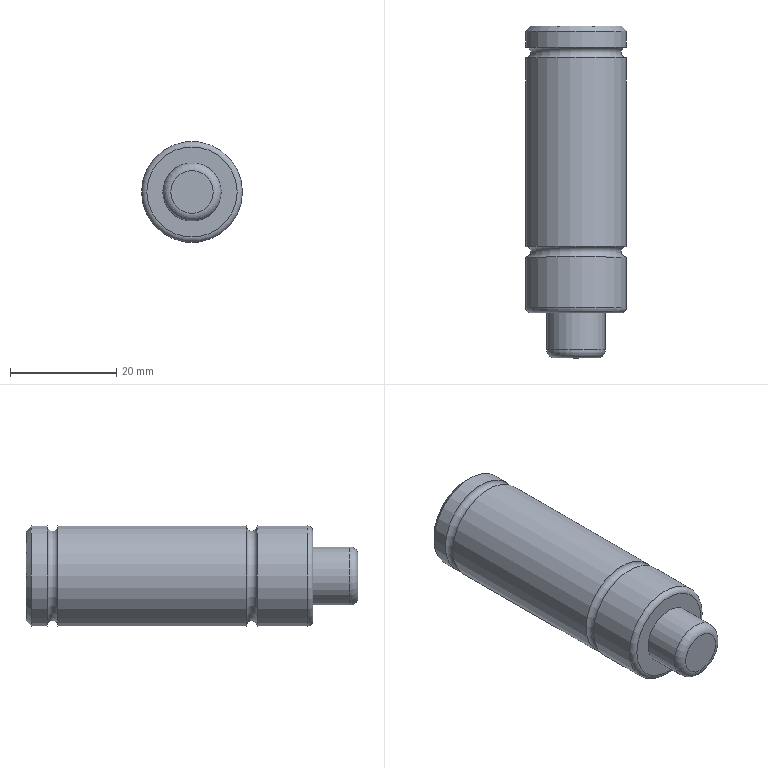Part | STEP file | 1_id602_x_t | 1 solid | 14 faces | box 19 x 62.5 x 19 mm | volume 15480 mm3 | cylinder 5 | torus 4 | plane 3 | cone 2 | commonest cylinder face diameters 19 x3 5 x1 11 x1
STEP:
#1=CARTESIAN_POINT('',(0.,0.,0.));
#2=DIRECTION('',(0.,0.,1.));
#3=DIRECTION('',(1.,0.,0.));
#4=AXIS2_PLACEMENT_3D('',#1,#2,#3);
#5=CARTESIAN_POINT('',(747.425,262.37,-108.684));
#6=VERTEX_POINT('',#5);
#7=CARTESIAN_POINT('',(752.425,262.37,-108.684));
#8=VERTEX_POINT('',#7);
#9=CARTESIAN_POINT('',(749.925,262.37,-108.684));
#10=DIRECTION('',(0.,1.,0.));
#11=DIRECTION('',(1.,0.,0.));
#12=AXIS2_PLACEMENT_3D('',#9,#10,#11);
#13=CIRCLE('',#12,2.5);
#14=CARTESIAN_POINT('',(749.925,261.669,-108.684));
#15=DIRECTION('',(0.,1.,0.));
#16=DIRECTION('',(-1.,0.,0.));
#17=AXIS2_PLACEMENT_3D('',#14,#15,#16);
#18=CONICAL_SURFACE('',#17,1.285,1.047);
#19=CARTESIAN_POINT('',(-3.142,0.7013));
#20=DIRECTION('',(1.,0.));
#21=VECTOR('',#20,1.);
#22=LINE('',#19,#21);
#23=(GEOMETRIC_REPRESENTATION_CONTEXT(2)PARAMETRIC_REPRESENTATION_CONTEXT()REPRESENTATION_CONTEXT('',''));
#24=DEFINITIONAL_REPRESENTATION('',(#22),#23);
#25=PCURVE('',#18,#24);
#26=CARTESIAN_POINT('',(749.925,262.37,-108.684));
#27=DIRECTION('',(0.,-1.,0.));
#28=DIRECTION('',(-1.,0.,0.));
#29=AXIS2_PLACEMENT_3D('',#26,#27,#28);
#30=CYLINDRICAL_SURFACE('',#29,2.5);
#31=CARTESIAN_POINT('',(9.425,0.));
#32=DIRECTION('',(-1.,0.));
#33=VECTOR('',#32,1.);
#34=LINE('',#31,#33);
#35=(GEOMETRIC_REPRESENTATION_CONTEXT(2)PARAMETRIC_REPRESENTATION_CONTEXT()REPRESENTATION_CONTEXT('',''));
#36=DEFINITIONAL_REPRESENTATION('',(#34),#35);
#37=PCURVE('',#30,#36);
#38=SURFACE_CURVE('',#13,(#25,#37),.PCURVE_S1.);
#39=EDGE_CURVE('',#6,#8,#38,.T.);
#40=ORIENTED_EDGE('',*,*,#39,.F.);
#41=CARTESIAN_POINT('',(749.925,260.927,-108.684));
#42=VERTEX_POINT('',#41);
#43=CARTESIAN_POINT('',(749.925,260.927,-108.684));
#44=CARTESIAN_POINT('',(747.425,262.37,-108.684));
#45=B_SPLINE_CURVE_WITH_KNOTS('',1,(#43,#44),.UNSPECIFIED.,.F.,.F.,(2,2),(-1.484,1.403),.PIECEWISE_BEZIER_KNOTS.);
#46=CARTESIAN_POINT('',(0.,0.));
#47=DIRECTION('',(0.,1.));
#48=VECTOR('',#47,1.);
#49=LINE('',#46,#48);
#50=(GEOMETRIC_REPRESENTATION_CONTEXT(2)PARAMETRIC_REPRESENTATION_CONTEXT()REPRESENTATION_CONTEXT('',''));
#51=DEFINITIONAL_REPRESENTATION('',(#49),#50);
#52=PCURVE('',#18,#51);
#53=CARTESIAN_POINT('',(6.283,0.));
#54=DIRECTION('',(0.,1.));
#55=VECTOR('',#54,1.);
#56=LINE('',#53,#55);
#57=(GEOMETRIC_REPRESENTATION_CONTEXT(2)PARAMETRIC_REPRESENTATION_CONTEXT()REPRESENTATION_CONTEXT('',''));
#58=DEFINITIONAL_REPRESENTATION('',(#56),#57);
#59=PCURVE('',#18,#58);
#60=SEAM_CURVE('',#45,(#52,#59),.PCURVE_S1.);
#61=EDGE_CURVE('',#42,#6,#60,.T.);
#62=ORIENTED_EDGE('',*,*,#61,.F.);
#63=ORIENTED_EDGE('',*,*,#61,.T.);
#64=CARTESIAN_POINT('',(749.925,262.37,-108.684));
#65=DIRECTION('',(0.,1.,0.));
#66=DIRECTION('',(1.,0.,0.));
#67=AXIS2_PLACEMENT_3D('',#64,#65,#66);
#68=CIRCLE('',#67,2.5);
#69=CARTESIAN_POINT('',(3.142,0.7013));
#70=DIRECTION('',(1.,0.));
#71=VECTOR('',#70,1.);
#72=LINE('',#69,#71);
#73=(GEOMETRIC_REPRESENTATION_CONTEXT(2)PARAMETRIC_REPRESENTATION_CONTEXT()REPRESENTATION_CONTEXT('',''));
#74=DEFINITIONAL_REPRESENTATION('',(#72),#73);
#75=PCURVE('',#18,#74);
#76=CARTESIAN_POINT('',(3.142,0.));
#77=DIRECTION('',(-1.,0.));
#78=VECTOR('',#77,1.);
#79=LINE('',#76,#78);
#80=(GEOMETRIC_REPRESENTATION_CONTEXT(2)PARAMETRIC_REPRESENTATION_CONTEXT()REPRESENTATION_CONTEXT('',''));
#81=DEFINITIONAL_REPRESENTATION('',(#79),#80);
#82=PCURVE('',#30,#81);
#83=SURFACE_CURVE('',#68,(#75,#82),.PCURVE_S1.);
#84=EDGE_CURVE('',#8,#6,#83,.T.);
#85=ORIENTED_EDGE('',*,*,#84,.F.);
#86=EDGE_LOOP('',(#40,#62,#63,#85));
#87=FACE_BOUND('',#86,.F.);
#88=ADVANCED_FACE('',(#87),#18,.F.);
#89=ORIENTED_EDGE('',*,*,#39,.T.);
#90=ORIENTED_EDGE('',*,*,#84,.T.);
#91=CARTESIAN_POINT('',(747.425,282.37,-108.684));
#92=VERTEX_POINT('',#91);
#93=CARTESIAN_POINT('',(747.425,282.37,-108.684));
#94=CARTESIAN_POINT('',(747.425,262.37,-108.684));
#95=B_SPLINE_CURVE_WITH_KNOTS('',1,(#93,#94),.UNSPECIFIED.,.F.,.F.,(2,2),(-20.,0.),.PIECEWISE_BEZIER_KNOTS.);
#96=CARTESIAN_POINT('',(0.,0.));
#97=DIRECTION('',(0.,1.));
#98=VECTOR('',#97,1.);
#99=LINE('',#96,#98);
#100=(GEOMETRIC_REPRESENTATION_CONTEXT(2)PARAMETRIC_REPRESENTATION_CONTEXT()REPRESENTATION_CONTEXT('',''));
#101=DEFINITIONAL_REPRESENTATION('',(#99),#100);
#102=PCURVE('',#30,#101);
#103=CARTESIAN_POINT('',(6.283,0.));
#104=DIRECTION('',(0.,1.));
#105=VECTOR('',#104,1.);
#106=LINE('',#103,#105);
#107=(GEOMETRIC_REPRESENTATION_CONTEXT(2)PARAMETRIC_REPRESENTATION_CONTEXT()REPRESENTATION_CONTEXT('',''));
#108=DEFINITIONAL_REPRESENTATION('',(#106),#107);
#109=PCURVE('',#30,#108);
#110=SEAM_CURVE('',#95,(#102,#109),.PCURVE_S1.);
#111=EDGE_CURVE('',#92,#6,#110,.T.);
#112=ORIENTED_EDGE('',*,*,#111,.F.);
#113=CARTESIAN_POINT('',(749.925,282.37,-108.684));
#114=DIRECTION('',(0.,-1.,0.));
#115=DIRECTION('',(-1.,0.,0.));
#116=AXIS2_PLACEMENT_3D('',#113,#114,#115);
#117=CIRCLE('',#116,2.5);
#118=CARTESIAN_POINT('',(0.,-20.));
#119=DIRECTION('',(1.,0.));
#120=VECTOR('',#119,1.);
#121=LINE('',#118,#120);
#122=(GEOMETRIC_REPRESENTATION_CONTEXT(2)PARAMETRIC_REPRESENTATION_CONTEXT()REPRESENTATION_CONTEXT('',''));
#123=DEFINITIONAL_REPRESENTATION('',(#121),#122);
#124=PCURVE('',#30,#123);
#125=CARTESIAN_POINT('',(749.925,282.37,-100.184));
#126=DIRECTION('',(0.,-1.,0.));
#127=DIRECTION('',(-1.,0.,0.));
#128=AXIS2_PLACEMENT_3D('',#125,#126,#127);
#129=PLANE('',#128);
#130=CARTESIAN_POINT('',(0.,8.5));
#131=DIRECTION('',(1.,0.));
#132=AXIS2_PLACEMENT_2D('',#130,#131);
#133=CIRCLE('',#132,2.5);
#134=(GEOMETRIC_REPRESENTATION_CONTEXT(2)PARAMETRIC_REPRESENTATION_CONTEXT()REPRESENTATION_CONTEXT('',''));
#135=DEFINITIONAL_REPRESENTATION('',(#133),#134);
#136=PCURVE('',#129,#135);
#137=SURFACE_CURVE('',#117,(#124,#136),.PCURVE_S1.);
#138=EDGE_CURVE('',#92,#92,#137,.T.);
#139=ORIENTED_EDGE('',*,*,#138,.T.);
#140=ORIENTED_EDGE('',*,*,#111,.T.);
#141=EDGE_LOOP('',(#89,#90,#112,#139,#140));
#142=FACE_BOUND('',#141,.F.);
#143=ADVANCED_FACE('',(#142),#30,.F.);
#144=CARTESIAN_POINT('',(758.425,282.37,-108.684));
#145=VERTEX_POINT('',#144);
#146=CARTESIAN_POINT('',(749.925,282.37,-108.684));
#147=DIRECTION('',(0.,1.,0.));
#148=DIRECTION('',(1.,0.,0.));
#149=AXIS2_PLACEMENT_3D('',#146,#147,#148);
#150=CIRCLE('',#149,8.5);
#151=CARTESIAN_POINT('',(-8.5,8.5));
#152=CARTESIAN_POINT('',(-8.5,23.222));
#153=CARTESIAN_POINT('',(4.25,15.861));
#154=CARTESIAN_POINT('',(17.,8.5));
#155=CARTESIAN_POINT('',(4.25,1.139));
#156=CARTESIAN_POINT('',(-8.5,-6.222));
#157=CARTESIAN_POINT('',(-8.5,8.5));
#158=(BOUNDED_CURVE()B_SPLINE_CURVE(2,(#151,#152,#153,#154,#155,#156,#157),.UNSPECIFIED.,.T.,.F.)B_SPLINE_CURVE_WITH_KNOTS((1,2,2,2,2,1),(-2.094,0.,2.094,4.189,6.283,8.378),.UNSPECIFIED.)CURVE()GEOMETRIC_REPRESENTATION_ITEM()RATIONAL_B_SPLINE_CURVE((1.,0.5,1.,0.5,1.,0.5,1.))REPRESENTATION_ITEM(''));
#159=(GEOMETRIC_REPRESENTATION_CONTEXT(2)PARAMETRIC_REPRESENTATION_CONTEXT()REPRESENTATION_CONTEXT('',''));
#160=DEFINITIONAL_REPRESENTATION('',(#158),#159);
#161=PCURVE('',#129,#160);
#162=CARTESIAN_POINT('',(749.925,281.87,-108.684));
#163=DIRECTION('',(0.,-1.,0.));
#164=DIRECTION('',(1.,0.,0.));
#165=AXIS2_PLACEMENT_3D('',#162,#163,#164);
#166=CONICAL_SURFACE('',#165,9.,0.7854);
#167=CARTESIAN_POINT('',(6.283,-0.5));
#168=DIRECTION('',(-1.,0.));
#169=VECTOR('',#168,1.);
#170=LINE('',#167,#169);
#171=(GEOMETRIC_REPRESENTATION_CONTEXT(2)PARAMETRIC_REPRESENTATION_CONTEXT()REPRESENTATION_CONTEXT('',''));
#172=DEFINITIONAL_REPRESENTATION('',(#170),#171);
#173=PCURVE('',#166,#172);
#174=SURFACE_CURVE('',#150,(#161,#173),.PCURVE_S1.);
#175=EDGE_CURVE('',#145,#145,#174,.T.);
#176=ORIENTED_EDGE('',*,*,#175,.T.);
#177=EDGE_LOOP('',(#176));
#178=FACE_BOUND('',#177,.T.);
#179=ORIENTED_EDGE('',*,*,#138,.T.);
#180=EDGE_LOOP('',(#179));
#181=FACE_BOUND('',#180,.T.);
#182=ADVANCED_FACE('',(#178,#181),#129,.F.);
#183=CARTESIAN_POINT('',(759.425,281.37,-108.684));
#184=VERTEX_POINT('',#183);
#185=CARTESIAN_POINT('',(740.425,281.37,-108.684));
#186=VERTEX_POINT('',#185);
#187=CARTESIAN_POINT('',(749.925,281.37,-108.684));
#188=DIRECTION('',(0.,1.,0.));
#189=DIRECTION('',(1.,0.,0.));
#190=AXIS2_PLACEMENT_3D('',#187,#188,#189);
#191=CIRCLE('',#190,9.5);
#192=CARTESIAN_POINT('',(6.283,0.5));
#193=DIRECTION('',(-1.,0.));
#194=VECTOR('',#193,1.);
#195=LINE('',#192,#194);
#196=(GEOMETRIC_REPRESENTATION_CONTEXT(2)PARAMETRIC_REPRESENTATION_CONTEXT()REPRESENTATION_CONTEXT('',''));
#197=DEFINITIONAL_REPRESENTATION('',(#195),#196);
#198=PCURVE('',#166,#197);
#199=CARTESIAN_POINT('',(749.925,228.37,-108.684));
#200=DIRECTION('',(0.,-1.,0.));
#201=DIRECTION('',(-1.,0.,0.));
#202=AXIS2_PLACEMENT_3D('',#199,#200,#201);
#203=CYLINDRICAL_SURFACE('',#202,9.5);
#204=CARTESIAN_POINT('',(3.142,-53.));
#205=DIRECTION('',(-1.,0.));
#206=VECTOR('',#205,1.);
#207=LINE('',#204,#206);
#208=(GEOMETRIC_REPRESENTATION_CONTEXT(2)PARAMETRIC_REPRESENTATION_CONTEXT()REPRESENTATION_CONTEXT('',''));
#209=DEFINITIONAL_REPRESENTATION('',(#207),#208);
#210=PCURVE('',#203,#209);
#211=SURFACE_CURVE('',#191,(#198,#210),.PCURVE_S1.);
#212=EDGE_CURVE('',#184,#186,#211,.T.);
#213=ORIENTED_EDGE('',*,*,#212,.T.);
#214=CARTESIAN_POINT('',(749.925,281.37,-108.684));
#215=DIRECTION('',(0.,1.,0.));
#216=DIRECTION('',(1.,0.,0.));
#217=AXIS2_PLACEMENT_3D('',#214,#215,#216);
#218=CIRCLE('',#217,9.5);
#219=CARTESIAN_POINT('',(6.283,0.5));
#220=DIRECTION('',(-1.,0.));
#221=VECTOR('',#220,1.);
#222=LINE('',#219,#221);
#223=(GEOMETRIC_REPRESENTATION_CONTEXT(2)PARAMETRIC_REPRESENTATION_CONTEXT()REPRESENTATION_CONTEXT('',''));
#224=DEFINITIONAL_REPRESENTATION('',(#222),#223);
#225=PCURVE('',#166,#224);
#226=CARTESIAN_POINT('',(9.425,-53.));
#227=DIRECTION('',(-1.,0.));
#228=VECTOR('',#227,1.);
#229=LINE('',#226,#228);
#230=(GEOMETRIC_REPRESENTATION_CONTEXT(2)PARAMETRIC_REPRESENTATION_CONTEXT()REPRESENTATION_CONTEXT('',''));
#231=DEFINITIONAL_REPRESENTATION('',(#229),#230);
#232=PCURVE('',#203,#231);
#233=SURFACE_CURVE('',#218,(#225,#232),.PCURVE_S1.);
#234=EDGE_CURVE('',#186,#184,#233,.T.);
#235=ORIENTED_EDGE('',*,*,#234,.T.);
#236=CARTESIAN_POINT('',(758.425,282.37,-108.684));
#237=CARTESIAN_POINT('',(759.425,281.37,-108.684));
#238=B_SPLINE_CURVE_WITH_KNOTS('',1,(#236,#237),.UNSPECIFIED.,.F.,.F.,(2,2),(-0.7071,0.7071),.PIECEWISE_BEZIER_KNOTS.);
#239=CARTESIAN_POINT('',(0.,0.));
#240=DIRECTION('',(0.,1.));
#241=VECTOR('',#240,1.);
#242=LINE('',#239,#241);
#243=(GEOMETRIC_REPRESENTATION_CONTEXT(2)PARAMETRIC_REPRESENTATION_CONTEXT()REPRESENTATION_CONTEXT('',''));
#244=DEFINITIONAL_REPRESENTATION('',(#242),#243);
#245=PCURVE('',#166,#244);
#246=CARTESIAN_POINT('',(6.283,0.));
#247=DIRECTION('',(0.,1.));
#248=VECTOR('',#247,1.);
#249=LINE('',#246,#248);
#250=(GEOMETRIC_REPRESENTATION_CONTEXT(2)PARAMETRIC_REPRESENTATION_CONTEXT()REPRESENTATION_CONTEXT('',''));
#251=DEFINITIONAL_REPRESENTATION('',(#249),#250);
#252=PCURVE('',#166,#251);
#253=SEAM_CURVE('',#238,(#245,#252),.PCURVE_S1.);
#254=EDGE_CURVE('',#145,#184,#253,.T.);
#255=ORIENTED_EDGE('',*,*,#254,.F.);
#256=ORIENTED_EDGE('',*,*,#175,.F.);
#257=ORIENTED_EDGE('',*,*,#254,.T.);
#258=EDGE_LOOP('',(#213,#235,#255,#256,#257));
#259=FACE_BOUND('',#258,.T.);
#260=ADVANCED_FACE('',(#259),#166,.T.);
#261=CARTESIAN_POINT('',(740.425,278.37,-108.684));
#262=VERTEX_POINT('',#261);
#263=CARTESIAN_POINT('',(749.925,278.37,-108.684));
#264=DIRECTION('',(0.,-1.,0.));
#265=DIRECTION('',(-1.,0.,0.));
#266=AXIS2_PLACEMENT_3D('',#263,#264,#265);
#267=CIRCLE('',#266,9.5);
#268=CARTESIAN_POINT('',(0.,-50.));
#269=DIRECTION('',(1.,0.));
#270=VECTOR('',#269,1.);
#271=LINE('',#268,#270);
#272=(GEOMETRIC_REPRESENTATION_CONTEXT(2)PARAMETRIC_REPRESENTATION_CONTEXT()REPRESENTATION_CONTEXT('',''));
#273=DEFINITIONAL_REPRESENTATION('',(#271),#272);
#274=PCURVE('',#203,#273);
#275=CARTESIAN_POINT('',(749.925,277.37,-108.684));
#276=DIRECTION('',(0.,1.,0.));
#277=DIRECTION('',(-1.,0.,0.));
#278=AXIS2_PLACEMENT_3D('',#275,#276,#277);
#279=TOROIDAL_SURFACE('',#278,9.5,1.);
#280=CARTESIAN_POINT('',(6.283,1.571));
#281=DIRECTION('',(-1.,0.));
#282=VECTOR('',#281,1.);
#283=LINE('',#280,#282);
#284=(GEOMETRIC_REPRESENTATION_CONTEXT(2)PARAMETRIC_REPRESENTATION_CONTEXT()REPRESENTATION_CONTEXT('',''));
#285=DEFINITIONAL_REPRESENTATION('',(#283),#284);
#286=PCURVE('',#279,#285);
#287=SURFACE_CURVE('',#267,(#274,#286),.PCURVE_S1.);
#288=EDGE_CURVE('',#262,#262,#287,.T.);
#289=ORIENTED_EDGE('',*,*,#288,.F.);
#290=CARTESIAN_POINT('',(740.425,281.37,-108.684));
#291=CARTESIAN_POINT('',(740.425,278.37,-108.684));
#292=B_SPLINE_CURVE_WITH_KNOTS('',1,(#290,#291),.UNSPECIFIED.,.F.,.F.,(2,2),(-53.,-50.),.PIECEWISE_BEZIER_KNOTS.);
#293=CARTESIAN_POINT('',(0.,0.));
#294=DIRECTION('',(0.,1.));
#295=VECTOR('',#294,1.);
#296=LINE('',#293,#295);
#297=(GEOMETRIC_REPRESENTATION_CONTEXT(2)PARAMETRIC_REPRESENTATION_CONTEXT()REPRESENTATION_CONTEXT('',''));
#298=DEFINITIONAL_REPRESENTATION('',(#296),#297);
#299=PCURVE('',#203,#298);
#300=CARTESIAN_POINT('',(6.283,0.));
#301=DIRECTION('',(0.,1.));
#302=VECTOR('',#301,1.);
#303=LINE('',#300,#302);
#304=(GEOMETRIC_REPRESENTATION_CONTEXT(2)PARAMETRIC_REPRESENTATION_CONTEXT()REPRESENTATION_CONTEXT('',''));
#305=DEFINITIONAL_REPRESENTATION('',(#303),#304);
#306=PCURVE('',#203,#305);
#307=SEAM_CURVE('',#292,(#299,#306),.PCURVE_S1.);
#308=EDGE_CURVE('',#186,#262,#307,.T.);
#309=ORIENTED_EDGE('',*,*,#308,.F.);
#310=ORIENTED_EDGE('',*,*,#212,.F.);
#311=ORIENTED_EDGE('',*,*,#234,.F.);
#312=ORIENTED_EDGE('',*,*,#308,.T.);
#313=EDGE_LOOP('',(#289,#309,#310,#311,#312));
#314=FACE_BOUND('',#313,.T.);
#315=ADVANCED_FACE('',(#314),#203,.T.);
#316=CARTESIAN_POINT('',(740.425,276.37,-108.684));
#317=VERTEX_POINT('',#316);
#318=CARTESIAN_POINT('',(749.925,276.37,-108.684));
#319=DIRECTION('',(0.,1.,0.));
#320=DIRECTION('',(-1.,0.,0.));
#321=AXIS2_PLACEMENT_3D('',#318,#319,#320);
#322=CIRCLE('',#321,9.5);
#323=CARTESIAN_POINT('',(0.,4.712));
#324=DIRECTION('',(1.,0.));
#325=VECTOR('',#324,1.);
#326=LINE('',#323,#325);
#327=(GEOMETRIC_REPRESENTATION_CONTEXT(2)PARAMETRIC_REPRESENTATION_CONTEXT()REPRESENTATION_CONTEXT('',''));
#328=DEFINITIONAL_REPRESENTATION('',(#326),#327);
#329=PCURVE('',#279,#328);
#330=CARTESIAN_POINT('',(749.925,228.37,-108.684));
#331=DIRECTION('',(0.,-1.,0.));
#332=DIRECTION('',(-1.,0.,0.));
#333=AXIS2_PLACEMENT_3D('',#330,#331,#332);
#334=CYLINDRICAL_SURFACE('',#333,9.5);
#335=CARTESIAN_POINT('',(6.283,-48.));
#336=DIRECTION('',(-1.,0.));
#337=VECTOR('',#336,1.);
#338=LINE('',#335,#337);
#339=(GEOMETRIC_REPRESENTATION_CONTEXT(2)PARAMETRIC_REPRESENTATION_CONTEXT()REPRESENTATION_CONTEXT('',''));
#340=DEFINITIONAL_REPRESENTATION('',(#338),#339);
#341=PCURVE('',#334,#340);
#342=SURFACE_CURVE('',#322,(#329,#341),.PCURVE_S1.);
#343=EDGE_CURVE('',#317,#317,#342,.T.);
#344=ORIENTED_EDGE('',*,*,#343,.F.);
#345=CARTESIAN_POINT('',(740.425,278.37,-108.684));
#346=CARTESIAN_POINT('',(740.818,278.37,-108.684));
#347=CARTESIAN_POINT('',(741.21,278.194,-108.684));
#348=CARTESIAN_POINT('',(741.511,277.841,-108.684));
#349=CARTESIAN_POINT('',(741.627,277.37,-108.684));
#350=CARTESIAN_POINT('',(741.511,276.899,-108.684));
#351=CARTESIAN_POINT('',(741.21,276.546,-108.684));
#352=CARTESIAN_POINT('',(740.818,276.37,-108.684));
#353=CARTESIAN_POINT('',(740.425,276.37,-108.684));
#354=B_SPLINE_CURVE_WITH_KNOTS('',8,(#345,#346,#347,#348,#349,#350,#351,#352,#353),.UNSPECIFIED.,.F.,.F.,(9,9),(1.571,4.712),.PIECEWISE_BEZIER_KNOTS.);
#355=CARTESIAN_POINT('',(0.,0.));
#356=DIRECTION('',(0.,1.));
#357=VECTOR('',#356,1.);
#358=LINE('',#355,#357);
#359=(GEOMETRIC_REPRESENTATION_CONTEXT(2)PARAMETRIC_REPRESENTATION_CONTEXT()REPRESENTATION_CONTEXT('',''));
#360=DEFINITIONAL_REPRESENTATION('',(#358),#359);
#361=PCURVE('',#279,#360);
#362=CARTESIAN_POINT('',(6.283,0.));
#363=DIRECTION('',(0.,1.));
#364=VECTOR('',#363,1.);
#365=LINE('',#362,#364);
#366=(GEOMETRIC_REPRESENTATION_CONTEXT(2)PARAMETRIC_REPRESENTATION_CONTEXT()REPRESENTATION_CONTEXT('',''));
#367=DEFINITIONAL_REPRESENTATION('',(#365),#366);
#368=PCURVE('',#279,#367);
#369=SEAM_CURVE('',#354,(#361,#368),.PCURVE_S1.);
#370=EDGE_CURVE('',#262,#317,#369,.T.);
#371=ORIENTED_EDGE('',*,*,#370,.F.);
#372=ORIENTED_EDGE('',*,*,#288,.F.);
#373=ORIENTED_EDGE('',*,*,#370,.T.);
#374=EDGE_LOOP('',(#344,#371,#372,#373));
#375=FACE_BOUND('',#374,.F.);
#376=ADVANCED_FACE('',(#375),#279,.F.);
#377=CARTESIAN_POINT('',(740.425,240.87,-108.684));
#378=VERTEX_POINT('',#377);
#379=CARTESIAN_POINT('',(759.425,240.87,-108.684));
#380=VERTEX_POINT('',#379);
#381=CARTESIAN_POINT('',(749.925,240.87,-108.684));
#382=DIRECTION('',(0.,-1.,0.));
#383=DIRECTION('',(1.,0.,0.));
#384=AXIS2_PLACEMENT_3D('',#381,#382,#383);
#385=CIRCLE('',#384,9.5);
#386=CARTESIAN_POINT('',(-3.142,-12.5));
#387=DIRECTION('',(1.,0.));
#388=VECTOR('',#387,1.);
#389=LINE('',#386,#388);
#390=(GEOMETRIC_REPRESENTATION_CONTEXT(2)PARAMETRIC_REPRESENTATION_CONTEXT()REPRESENTATION_CONTEXT('',''));
#391=DEFINITIONAL_REPRESENTATION('',(#389),#390);
#392=PCURVE('',#334,#391);
#393=CARTESIAN_POINT('',(749.925,239.87,-108.684));
#394=DIRECTION('',(0.,1.,0.));
#395=DIRECTION('',(-1.,0.,0.));
#396=AXIS2_PLACEMENT_3D('',#393,#394,#395);
#397=TOROIDAL_SURFACE('',#396,9.5,1.);
#398=CARTESIAN_POINT('',(9.425,1.571));
#399=DIRECTION('',(-1.,0.));
#400=VECTOR('',#399,1.);
#401=LINE('',#398,#400);
#402=(GEOMETRIC_REPRESENTATION_CONTEXT(2)PARAMETRIC_REPRESENTATION_CONTEXT()REPRESENTATION_CONTEXT('',''));
#403=DEFINITIONAL_REPRESENTATION('',(#401),#402);
#404=PCURVE('',#397,#403);
#405=SURFACE_CURVE('',#385,(#392,#404),.PCURVE_S1.);
#406=EDGE_CURVE('',#378,#380,#405,.T.);
#407=ORIENTED_EDGE('',*,*,#406,.F.);
#408=CARTESIAN_POINT('',(740.425,276.37,-108.684));
#409=CARTESIAN_POINT('',(740.425,240.87,-108.684));
#410=B_SPLINE_CURVE_WITH_KNOTS('',1,(#408,#409),.UNSPECIFIED.,.F.,.F.,(2,2),(-48.,-12.5),.PIECEWISE_BEZIER_KNOTS.);
#411=CARTESIAN_POINT('',(0.,0.));
#412=DIRECTION('',(0.,1.));
#413=VECTOR('',#412,1.);
#414=LINE('',#411,#413);
#415=(GEOMETRIC_REPRESENTATION_CONTEXT(2)PARAMETRIC_REPRESENTATION_CONTEXT()REPRESENTATION_CONTEXT('',''));
#416=DEFINITIONAL_REPRESENTATION('',(#414),#415);
#417=PCURVE('',#334,#416);
#418=CARTESIAN_POINT('',(6.283,0.));
#419=DIRECTION('',(0.,1.));
#420=VECTOR('',#419,1.);
#421=LINE('',#418,#420);
#422=(GEOMETRIC_REPRESENTATION_CONTEXT(2)PARAMETRIC_REPRESENTATION_CONTEXT()REPRESENTATION_CONTEXT('',''));
#423=DEFINITIONAL_REPRESENTATION('',(#421),#422);
#424=PCURVE('',#334,#423);
#425=SEAM_CURVE('',#410,(#417,#424),.PCURVE_S1.);
#426=EDGE_CURVE('',#317,#378,#425,.T.);
#427=ORIENTED_EDGE('',*,*,#426,.F.);
#428=ORIENTED_EDGE('',*,*,#343,.F.);
#429=ORIENTED_EDGE('',*,*,#426,.T.);
#430=CARTESIAN_POINT('',(749.925,240.87,-108.684));
#431=DIRECTION('',(0.,-1.,0.));
#432=DIRECTION('',(1.,0.,0.));
#433=AXIS2_PLACEMENT_3D('',#430,#431,#432);
#434=CIRCLE('',#433,9.5);
#435=CARTESIAN_POINT('',(3.142,-12.5));
#436=DIRECTION('',(1.,0.));
#437=VECTOR('',#436,1.);
#438=LINE('',#435,#437);
#439=(GEOMETRIC_REPRESENTATION_CONTEXT(2)PARAMETRIC_REPRESENTATION_CONTEXT()REPRESENTATION_CONTEXT('',''));
#440=DEFINITIONAL_REPRESENTATION('',(#438),#439);
#441=PCURVE('',#334,#440);
#442=CARTESIAN_POINT('',(9.425,1.571));
#443=DIRECTION('',(-1.,0.));
#444=VECTOR('',#443,1.);
#445=LINE('',#442,#444);
#446=(GEOMETRIC_REPRESENTATION_CONTEXT(2)PARAMETRIC_REPRESENTATION_CONTEXT()REPRESENTATION_CONTEXT('',''));
#447=DEFINITIONAL_REPRESENTATION('',(#445),#446);
#448=PCURVE('',#397,#447);
#449=SURFACE_CURVE('',#434,(#441,#448),.PCURVE_S1.);
#450=EDGE_CURVE('',#380,#378,#449,.T.);
#451=ORIENTED_EDGE('',*,*,#450,.F.);
#452=EDGE_LOOP('',(#407,#427,#428,#429,#451));
#453=FACE_BOUND('',#452,.T.);
#454=ADVANCED_FACE('',(#453),#334,.T.);
#455=CARTESIAN_POINT('',(759.425,238.87,-108.684));
#456=VERTEX_POINT('',#455);
#457=CARTESIAN_POINT('',(740.425,238.87,-108.684));
#458=VERTEX_POINT('',#457);
#459=CARTESIAN_POINT('',(749.925,238.87,-108.684));
#460=DIRECTION('',(0.,1.,0.));
#461=DIRECTION('',(1.,0.,0.));
#462=AXIS2_PLACEMENT_3D('',#459,#460,#461);
#463=CIRCLE('',#462,9.5);
#464=CARTESIAN_POINT('',(3.142,4.712));
#465=DIRECTION('',(1.,0.));
#466=VECTOR('',#465,1.);
#467=LINE('',#464,#466);
#468=(GEOMETRIC_REPRESENTATION_CONTEXT(2)PARAMETRIC_REPRESENTATION_CONTEXT()REPRESENTATION_CONTEXT('',''));
#469=DEFINITIONAL_REPRESENTATION('',(#467),#468);
#470=PCURVE('',#397,#469);
#471=CARTESIAN_POINT('',(749.925,228.37,-108.684));
#472=DIRECTION('',(0.,-1.,0.));
#473=DIRECTION('',(-1.,0.,0.));
#474=AXIS2_PLACEMENT_3D('',#471,#472,#473);
#475=CYLINDRICAL_SURFACE('',#474,9.5);
#476=CARTESIAN_POINT('',(3.142,-10.5));
#477=DIRECTION('',(-1.,0.));
#478=VECTOR('',#477,1.);
#479=LINE('',#476,#478);
#480=(GEOMETRIC_REPRESENTATION_CONTEXT(2)PARAMETRIC_REPRESENTATION_CONTEXT()REPRESENTATION_CONTEXT('',''));
#481=DEFINITIONAL_REPRESENTATION('',(#479),#480);
#482=PCURVE('',#475,#481);
#483=SURFACE_CURVE('',#463,(#470,#482),.PCURVE_S1.);
#484=EDGE_CURVE('',#456,#458,#483,.T.);
#485=ORIENTED_EDGE('',*,*,#484,.F.);
#486=CARTESIAN_POINT('',(759.425,240.87,-108.684));
#487=CARTESIAN_POINT('',(759.032,240.87,-108.684));
#488=CARTESIAN_POINT('',(758.64,240.694,-108.684));
#489=CARTESIAN_POINT('',(758.339,240.341,-108.684));
#490=CARTESIAN_POINT('',(758.223,239.87,-108.684));
#491=CARTESIAN_POINT('',(758.339,239.399,-108.684));
#492=CARTESIAN_POINT('',(758.64,239.046,-108.684));
#493=CARTESIAN_POINT('',(759.032,238.87,-108.684));
#494=CARTESIAN_POINT('',(759.425,238.87,-108.684));
#495=B_SPLINE_CURVE_WITH_KNOTS('',8,(#486,#487,#488,#489,#490,#491,#492,#493,#494),.UNSPECIFIED.,.F.,.F.,(9,9),(1.571,4.712),.PIECEWISE_BEZIER_KNOTS.);
#496=CARTESIAN_POINT('',(3.142,0.));
#497=DIRECTION('',(0.,1.));
#498=VECTOR('',#497,1.);
#499=LINE('',#496,#498);
#500=(GEOMETRIC_REPRESENTATION_CONTEXT(2)PARAMETRIC_REPRESENTATION_CONTEXT()REPRESENTATION_CONTEXT('',''));
#501=DEFINITIONAL_REPRESENTATION('',(#499),#500);
#502=PCURVE('',#397,#501);
#503=CARTESIAN_POINT('',(9.425,0.));
#504=DIRECTION('',(0.,1.));
#505=VECTOR('',#504,1.);
#506=LINE('',#503,#505);
#507=(GEOMETRIC_REPRESENTATION_CONTEXT(2)PARAMETRIC_REPRESENTATION_CONTEXT()REPRESENTATION_CONTEXT('',''));
#508=DEFINITIONAL_REPRESENTATION('',(#506),#507);
#509=PCURVE('',#397,#508);
#510=SEAM_CURVE('',#495,(#502,#509),.PCURVE_S1.);
#511=EDGE_CURVE('',#380,#456,#510,.T.);
#512=ORIENTED_EDGE('',*,*,#511,.F.);
#513=ORIENTED_EDGE('',*,*,#406,.F.);
#514=ORIENTED_EDGE('',*,*,#450,.F.);
#515=ORIENTED_EDGE('',*,*,#511,.T.);
#516=CARTESIAN_POINT('',(749.925,238.87,-108.684));
#517=DIRECTION('',(0.,1.,0.));
#518=DIRECTION('',(1.,0.,0.));
#519=AXIS2_PLACEMENT_3D('',#516,#517,#518);
#520=CIRCLE('',#519,9.5);
#521=CARTESIAN_POINT('',(3.142,4.712));
#522=DIRECTION('',(1.,0.));
#523=VECTOR('',#522,1.);
#524=LINE('',#521,#523);
#525=(GEOMETRIC_REPRESENTATION_CONTEXT(2)PARAMETRIC_REPRESENTATION_CONTEXT()REPRESENTATION_CONTEXT('',''));
#526=DEFINITIONAL_REPRESENTATION('',(#524),#525);
#527=PCURVE('',#397,#526);
#528=CARTESIAN_POINT('',(9.425,-10.5));
#529=DIRECTION('',(-1.,0.));
#530=VECTOR('',#529,1.);
#531=LINE('',#528,#530);
#532=(GEOMETRIC_REPRESENTATION_CONTEXT(2)PARAMETRIC_REPRESENTATION_CONTEXT()REPRESENTATION_CONTEXT('',''));
#533=DEFINITIONAL_REPRESENTATION('',(#531),#532);
#534=PCURVE('',#475,#533);
#535=SURFACE_CURVE('',#520,(#527,#534),.PCURVE_S1.);
#536=EDGE_CURVE('',#458,#456,#535,.T.);
#537=ORIENTED_EDGE('',*,*,#536,.F.);
#538=EDGE_LOOP('',(#485,#512,#513,#514,#515,#537));
#539=FACE_BOUND('',#538,.F.);
#540=ADVANCED_FACE('',(#539),#397,.F.);
#541=CARTESIAN_POINT('',(740.425,229.37,-108.684));
#542=VERTEX_POINT('',#541);
#543=CARTESIAN_POINT('',(749.925,229.37,-108.684));
#544=DIRECTION('',(0.,-1.,0.));
#545=DIRECTION('',(-1.,0.,0.));
#546=AXIS2_PLACEMENT_3D('',#543,#544,#545);
#547=CIRCLE('',#546,9.5);
#548=CARTESIAN_POINT('',(0.,-1.));
#549=DIRECTION('',(1.,0.));
#550=VECTOR('',#549,1.);
#551=LINE('',#548,#550);
#552=(GEOMETRIC_REPRESENTATION_CONTEXT(2)PARAMETRIC_REPRESENTATION_CONTEXT()REPRESENTATION_CONTEXT('',''));
#553=DEFINITIONAL_REPRESENTATION('',(#551),#552);
#554=PCURVE('',#475,#553);
#555=CARTESIAN_POINT('',(749.925,229.37,-108.684));
#556=DIRECTION('',(0.,1.,0.));
#557=DIRECTION('',(-1.,0.,0.));
#558=AXIS2_PLACEMENT_3D('',#555,#556,#557);
#559=TOROIDAL_SURFACE('',#558,8.5,1.);
#560=CARTESIAN_POINT('',(6.283,6.283));
#561=DIRECTION('',(-1.,0.));
#562=VECTOR('',#561,1.);
#563=LINE('',#560,#562);
#564=(GEOMETRIC_REPRESENTATION_CONTEXT(2)PARAMETRIC_REPRESENTATION_CONTEXT()REPRESENTATION_CONTEXT('',''));
#565=DEFINITIONAL_REPRESENTATION('',(#563),#564);
#566=PCURVE('',#559,#565);
#567=SURFACE_CURVE('',#547,(#554,#566),.PCURVE_S1.);
#568=EDGE_CURVE('',#542,#542,#567,.T.);
#569=ORIENTED_EDGE('',*,*,#568,.F.);
#570=CARTESIAN_POINT('',(740.425,238.87,-108.684));
#571=CARTESIAN_POINT('',(740.425,229.37,-108.684));
#572=B_SPLINE_CURVE_WITH_KNOTS('',1,(#570,#571),.UNSPECIFIED.,.F.,.F.,(2,2),(-10.5,-1.),.PIECEWISE_BEZIER_KNOTS.);
#573=CARTESIAN_POINT('',(0.,0.));
#574=DIRECTION('',(0.,1.));
#575=VECTOR('',#574,1.);
#576=LINE('',#573,#575);
#577=(GEOMETRIC_REPRESENTATION_CONTEXT(2)PARAMETRIC_REPRESENTATION_CONTEXT()REPRESENTATION_CONTEXT('',''));
#578=DEFINITIONAL_REPRESENTATION('',(#576),#577);
#579=PCURVE('',#475,#578);
#580=CARTESIAN_POINT('',(6.283,0.));
#581=DIRECTION('',(0.,1.));
#582=VECTOR('',#581,1.);
#583=LINE('',#580,#582);
#584=(GEOMETRIC_REPRESENTATION_CONTEXT(2)PARAMETRIC_REPRESENTATION_CONTEXT()REPRESENTATION_CONTEXT('',''));
#585=DEFINITIONAL_REPRESENTATION('',(#583),#584);
#586=PCURVE('',#475,#585);
#587=SEAM_CURVE('',#572,(#579,#586),.PCURVE_S1.);
#588=EDGE_CURVE('',#458,#542,#587,.T.);
#589=ORIENTED_EDGE('',*,*,#588,.F.);
#590=ORIENTED_EDGE('',*,*,#484,.F.);
#591=ORIENTED_EDGE('',*,*,#536,.F.);
#592=ORIENTED_EDGE('',*,*,#588,.T.);
#593=EDGE_LOOP('',(#569,#589,#590,#591,#592));
#594=FACE_BOUND('',#593,.T.);
#595=ADVANCED_FACE('',(#594),#475,.T.);
#596=ORIENTED_EDGE('',*,*,#568,.T.);
#597=CARTESIAN_POINT('',(741.425,228.37,-108.684));
#598=VERTEX_POINT('',#597);
#599=CARTESIAN_POINT('',(741.425,228.37,-108.684));
#600=CARTESIAN_POINT('',(741.158,228.37,-108.684));
#601=CARTESIAN_POINT('',(740.897,228.455,-108.684));
#602=CARTESIAN_POINT('',(740.673,228.618,-108.684));
#603=CARTESIAN_POINT('',(740.51,228.842,-108.684));
#604=CARTESIAN_POINT('',(740.425,229.103,-108.684));
#605=CARTESIAN_POINT('',(740.425,229.37,-108.684));
#606=(BOUNDED_CURVE()B_SPLINE_CURVE(6,(#599,#600,#601,#602,#603,#604,#605),.UNSPECIFIED.,.F.,.F.)B_SPLINE_CURVE_WITH_KNOTS((7,7),(-1.571,0.),.PIECEWISE_BEZIER_KNOTS.)CURVE()GEOMETRIC_REPRESENTATION_ITEM()RATIONAL_B_SPLINE_CURVE((1.031,1.01,0.9979,0.994,0.9979,1.01,1.031))REPRESENTATION_ITEM(''));
#607=CARTESIAN_POINT('',(0.,6.283));
#608=DIRECTION('',(0.,1.));
#609=VECTOR('',#608,1.);
#610=LINE('',#607,#609);
#611=(GEOMETRIC_REPRESENTATION_CONTEXT(2)PARAMETRIC_REPRESENTATION_CONTEXT()REPRESENTATION_CONTEXT('',''));
#612=DEFINITIONAL_REPRESENTATION('',(#610),#611);
#613=PCURVE('',#559,#612);
#614=CARTESIAN_POINT('',(6.283,6.283));
#615=DIRECTION('',(0.,1.));
#616=VECTOR('',#615,1.);
#617=LINE('',#614,#616);
#618=(GEOMETRIC_REPRESENTATION_CONTEXT(2)PARAMETRIC_REPRESENTATION_CONTEXT()REPRESENTATION_CONTEXT('',''));
#619=DEFINITIONAL_REPRESENTATION('',(#617),#618);
#620=PCURVE('',#559,#619);
#621=SEAM_CURVE('',#606,(#613,#620),.PCURVE_S1.);
#622=EDGE_CURVE('',#598,#542,#621,.T.);
#623=ORIENTED_EDGE('',*,*,#622,.F.);
#624=CARTESIAN_POINT('',(758.425,228.37,-108.684));
#625=VERTEX_POINT('',#624);
#626=CARTESIAN_POINT('',(749.925,228.37,-108.684));
#627=DIRECTION('',(0.,-1.,0.));
#628=DIRECTION('',(1.,0.,0.));
#629=AXIS2_PLACEMENT_3D('',#626,#627,#628);
#630=CIRCLE('',#629,8.5);
#631=CARTESIAN_POINT('',(3.142,4.712));
#632=DIRECTION('',(-1.,0.));
#633=VECTOR('',#632,1.);
#634=LINE('',#631,#633);
#635=(GEOMETRIC_REPRESENTATION_CONTEXT(2)PARAMETRIC_REPRESENTATION_CONTEXT()REPRESENTATION_CONTEXT('',''));
#636=DEFINITIONAL_REPRESENTATION('',(#634),#635);
#637=PCURVE('',#559,#636);
#638=CARTESIAN_POINT('',(749.925,228.37,-103.184));
#639=DIRECTION('',(0.,1.,0.));
#640=DIRECTION('',(1.,0.,0.));
#641=AXIS2_PLACEMENT_3D('',#638,#639,#640);
#642=PLANE('',#641);
#643=CARTESIAN_POINT('',(8.5,5.5));
#644=CARTESIAN_POINT('',(8.5,-9.222));
#645=CARTESIAN_POINT('',(-4.25,-1.861));
#646=CARTESIAN_POINT('',(-17.,5.5));
#647=CARTESIAN_POINT('',(-4.25,12.861));
#648=CARTESIAN_POINT('',(8.5,20.222));
#649=CARTESIAN_POINT('',(8.5,5.5));
#650=(BOUNDED_CURVE()B_SPLINE_CURVE(2,(#643,#644,#645,#646,#647,#648,#649),.UNSPECIFIED.,.T.,.F.)B_SPLINE_CURVE_WITH_KNOTS((1,2,2,2,2,1),(-2.094,0.,2.094,4.189,6.283,8.378),.UNSPECIFIED.)CURVE()GEOMETRIC_REPRESENTATION_ITEM()RATIONAL_B_SPLINE_CURVE((1.,0.5,1.,0.5,1.,0.5,1.))REPRESENTATION_ITEM(''));
#651=(GEOMETRIC_REPRESENTATION_CONTEXT(2)PARAMETRIC_REPRESENTATION_CONTEXT()REPRESENTATION_CONTEXT('',''));
#652=DEFINITIONAL_REPRESENTATION('',(#650),#651);
#653=PCURVE('',#642,#652);
#654=SURFACE_CURVE('',#630,(#637,#653),.PCURVE_S1.);
#655=EDGE_CURVE('',#625,#598,#654,.T.);
#656=ORIENTED_EDGE('',*,*,#655,.F.);
#657=CARTESIAN_POINT('',(749.925,228.37,-108.684));
#658=DIRECTION('',(0.,-1.,0.));
#659=DIRECTION('',(1.,0.,0.));
#660=AXIS2_PLACEMENT_3D('',#657,#658,#659);
#661=CIRCLE('',#660,8.5);
#662=CARTESIAN_POINT('',(9.425,4.712));
#663=DIRECTION('',(-1.,0.));
#664=VECTOR('',#663,1.);
#665=LINE('',#662,#664);
#666=(GEOMETRIC_REPRESENTATION_CONTEXT(2)PARAMETRIC_REPRESENTATION_CONTEXT()REPRESENTATION_CONTEXT('',''));
#667=DEFINITIONAL_REPRESENTATION('',(#665),#666);
#668=PCURVE('',#559,#667);
#669=CARTESIAN_POINT('',(8.5,5.5));
#670=CARTESIAN_POINT('',(8.5,-9.222));
#671=CARTESIAN_POINT('',(-4.25,-1.861));
#672=CARTESIAN_POINT('',(-17.,5.5));
#673=CARTESIAN_POINT('',(-4.25,12.861));
#674=CARTESIAN_POINT('',(8.5,20.222));
#675=CARTESIAN_POINT('',(8.5,5.5));
#676=(BOUNDED_CURVE()B_SPLINE_CURVE(2,(#669,#670,#671,#672,#673,#674,#675),.UNSPECIFIED.,.T.,.F.)B_SPLINE_CURVE_WITH_KNOTS((1,2,2,2,2,1),(-2.094,0.,2.094,4.189,6.283,8.378),.UNSPECIFIED.)CURVE()GEOMETRIC_REPRESENTATION_ITEM()RATIONAL_B_SPLINE_CURVE((1.,0.5,1.,0.5,1.,0.5,1.))REPRESENTATION_ITEM(''));
#677=(GEOMETRIC_REPRESENTATION_CONTEXT(2)PARAMETRIC_REPRESENTATION_CONTEXT()REPRESENTATION_CONTEXT('',''));
#678=DEFINITIONAL_REPRESENTATION('',(#676),#677);
#679=PCURVE('',#642,#678);
#680=SURFACE_CURVE('',#661,(#668,#679),.PCURVE_S1.);
#681=EDGE_CURVE('',#598,#625,#680,.T.);
#682=ORIENTED_EDGE('',*,*,#681,.F.);
#683=ORIENTED_EDGE('',*,*,#622,.T.);
#684=EDGE_LOOP('',(#596,#623,#656,#682,#683));
#685=FACE_BOUND('',#684,.T.);
#686=ADVANCED_FACE('',(#685),#559,.T.);
#687=ORIENTED_EDGE('',*,*,#655,.T.);
#688=ORIENTED_EDGE('',*,*,#681,.T.);
#689=EDGE_LOOP('',(#687,#688));
#690=FACE_BOUND('',#689,.T.);
#691=CARTESIAN_POINT('',(755.425,228.37,-108.684));
#692=VERTEX_POINT('',#691);
#693=CARTESIAN_POINT('',(744.425,228.37,-108.684));
#694=VERTEX_POINT('',#693);
#695=CARTESIAN_POINT('',(749.925,228.37,-108.684));
#696=DIRECTION('',(0.,1.,0.));
#697=DIRECTION('',(1.,0.,0.));
#698=AXIS2_PLACEMENT_3D('',#695,#696,#697);
#699=CIRCLE('',#698,5.5);
#700=CARTESIAN_POINT('',(0.,5.5));
#701=DIRECTION('',(1.,0.));
#702=AXIS2_PLACEMENT_2D('',#700,#701);
#703=CIRCLE('',#702,5.5);
#704=(GEOMETRIC_REPRESENTATION_CONTEXT(2)PARAMETRIC_REPRESENTATION_CONTEXT()REPRESENTATION_CONTEXT('',''));
#705=DEFINITIONAL_REPRESENTATION('',(#703),#704);
#706=PCURVE('',#642,#705);
#707=CARTESIAN_POINT('',(749.925,226.87,-108.684));
#708=DIRECTION('',(0.,-1.,0.));
#709=DIRECTION('',(-1.,0.,0.));
#710=AXIS2_PLACEMENT_3D('',#707,#708,#709);
#711=CYLINDRICAL_SURFACE('',#710,5.5);
#712=CARTESIAN_POINT('',(3.142,-1.5));
#713=DIRECTION('',(-1.,0.));
#714=VECTOR('',#713,1.);
#715=LINE('',#712,#714);
#716=(GEOMETRIC_REPRESENTATION_CONTEXT(2)PARAMETRIC_REPRESENTATION_CONTEXT()REPRESENTATION_CONTEXT('',''));
#717=DEFINITIONAL_REPRESENTATION('',(#715),#716);
#718=PCURVE('',#711,#717);
#719=SURFACE_CURVE('',#699,(#706,#718),.PCURVE_S1.);
#720=EDGE_CURVE('',#692,#694,#719,.T.);
#721=ORIENTED_EDGE('',*,*,#720,.T.);
#722=CARTESIAN_POINT('',(749.925,228.37,-108.684));
#723=DIRECTION('',(0.,1.,0.));
#724=DIRECTION('',(1.,0.,0.));
#725=AXIS2_PLACEMENT_3D('',#722,#723,#724);
#726=CIRCLE('',#725,5.5);
#727=CARTESIAN_POINT('',(0.,5.5));
#728=DIRECTION('',(1.,0.));
#729=AXIS2_PLACEMENT_2D('',#727,#728);
#730=CIRCLE('',#729,5.5);
#731=(GEOMETRIC_REPRESENTATION_CONTEXT(2)PARAMETRIC_REPRESENTATION_CONTEXT()REPRESENTATION_CONTEXT('',''));
#732=DEFINITIONAL_REPRESENTATION('',(#730),#731);
#733=PCURVE('',#642,#732);
#734=CARTESIAN_POINT('',(9.425,-1.5));
#735=DIRECTION('',(-1.,0.));
#736=VECTOR('',#735,1.);
#737=LINE('',#734,#736);
#738=(GEOMETRIC_REPRESENTATION_CONTEXT(2)PARAMETRIC_REPRESENTATION_CONTEXT()REPRESENTATION_CONTEXT('',''));
#739=DEFINITIONAL_REPRESENTATION('',(#737),#738);
#740=PCURVE('',#711,#739);
#741=SURFACE_CURVE('',#726,(#733,#740),.PCURVE_S1.);
#742=EDGE_CURVE('',#694,#692,#741,.T.);
#743=ORIENTED_EDGE('',*,*,#742,.T.);
#744=EDGE_LOOP('',(#721,#743));
#745=FACE_BOUND('',#744,.T.);
#746=ADVANCED_FACE('',(#690,#745),#642,.F.);
#747=CARTESIAN_POINT('',(744.425,221.37,-108.684));
#748=VERTEX_POINT('',#747);
#749=CARTESIAN_POINT('',(749.925,221.37,-108.684));
#750=DIRECTION('',(0.,-1.,0.));
#751=DIRECTION('',(-1.,0.,0.));
#752=AXIS2_PLACEMENT_3D('',#749,#750,#751);
#753=CIRCLE('',#752,5.5);
#754=CARTESIAN_POINT('',(0.,5.5));
#755=DIRECTION('',(1.,0.));
#756=VECTOR('',#755,1.);
#757=LINE('',#754,#756);
#758=(GEOMETRIC_REPRESENTATION_CONTEXT(2)PARAMETRIC_REPRESENTATION_CONTEXT()REPRESENTATION_CONTEXT('',''));
#759=DEFINITIONAL_REPRESENTATION('',(#757),#758);
#760=PCURVE('',#711,#759);
#761=CARTESIAN_POINT('',(749.925,221.37,-108.684));
#762=DIRECTION('',(0.,1.,0.));
#763=DIRECTION('',(-1.,0.,0.));
#764=AXIS2_PLACEMENT_3D('',#761,#762,#763);
#765=TOROIDAL_SURFACE('',#764,4.,1.5);
#766=CARTESIAN_POINT('',(6.283,6.283));
#767=DIRECTION('',(-1.,0.));
#768=VECTOR('',#767,1.);
#769=LINE('',#766,#768);
#770=(GEOMETRIC_REPRESENTATION_CONTEXT(2)PARAMETRIC_REPRESENTATION_CONTEXT()REPRESENTATION_CONTEXT('',''));
#771=DEFINITIONAL_REPRESENTATION('',(#769),#770);
#772=PCURVE('',#765,#771);
#773=SURFACE_CURVE('',#753,(#760,#772),.PCURVE_S1.);
#774=EDGE_CURVE('',#748,#748,#773,.T.);
#775=ORIENTED_EDGE('',*,*,#774,.F.);
#776=CARTESIAN_POINT('',(744.425,228.37,-108.684));
#777=CARTESIAN_POINT('',(744.425,221.37,-108.684));
#778=B_SPLINE_CURVE_WITH_KNOTS('',1,(#776,#777),.UNSPECIFIED.,.F.,.F.,(2,2),(-1.5,5.5),.PIECEWISE_BEZIER_KNOTS.);
#779=CARTESIAN_POINT('',(0.,0.));
#780=DIRECTION('',(0.,1.));
#781=VECTOR('',#780,1.);
#782=LINE('',#779,#781);
#783=(GEOMETRIC_REPRESENTATION_CONTEXT(2)PARAMETRIC_REPRESENTATION_CONTEXT()REPRESENTATION_CONTEXT('',''));
#784=DEFINITIONAL_REPRESENTATION('',(#782),#783);
#785=PCURVE('',#711,#784);
#786=CARTESIAN_POINT('',(6.283,0.));
#787=DIRECTION('',(0.,1.));
#788=VECTOR('',#787,1.);
#789=LINE('',#786,#788);
#790=(GEOMETRIC_REPRESENTATION_CONTEXT(2)PARAMETRIC_REPRESENTATION_CONTEXT()REPRESENTATION_CONTEXT('',''));
#791=DEFINITIONAL_REPRESENTATION('',(#789),#790);
#792=PCURVE('',#711,#791);
#793=SEAM_CURVE('',#778,(#785,#792),.PCURVE_S1.);
#794=EDGE_CURVE('',#694,#748,#793,.T.);
#795=ORIENTED_EDGE('',*,*,#794,.F.);
#796=ORIENTED_EDGE('',*,*,#720,.F.);
#797=ORIENTED_EDGE('',*,*,#742,.F.);
#798=ORIENTED_EDGE('',*,*,#794,.T.);
#799=EDGE_LOOP('',(#775,#795,#796,#797,#798));
#800=FACE_BOUND('',#799,.T.);
#801=ADVANCED_FACE('',(#800),#711,.T.);
#802=ORIENTED_EDGE('',*,*,#774,.T.);
#803=CARTESIAN_POINT('',(745.925,219.87,-108.684));
#804=VERTEX_POINT('',#803);
#805=CARTESIAN_POINT('',(745.925,219.87,-108.684));
#806=CARTESIAN_POINT('',(745.524,219.87,-108.684));
#807=CARTESIAN_POINT('',(745.133,219.997,-108.684));
#808=CARTESIAN_POINT('',(744.797,220.242,-108.684));
#809=CARTESIAN_POINT('',(744.553,220.578,-108.684));
#810=CARTESIAN_POINT('',(744.425,220.969,-108.684));
#811=CARTESIAN_POINT('',(744.425,221.37,-108.684));
#812=(BOUNDED_CURVE()B_SPLINE_CURVE(6,(#805,#806,#807,#808,#809,#810,#811),.UNSPECIFIED.,.F.,.F.)B_SPLINE_CURVE_WITH_KNOTS((7,7),(-1.571,0.),.PIECEWISE_BEZIER_KNOTS.)CURVE()GEOMETRIC_REPRESENTATION_ITEM()RATIONAL_B_SPLINE_CURVE((1.031,1.01,0.9979,0.994,0.9979,1.01,1.031))REPRESENTATION_ITEM(''));
#813=CARTESIAN_POINT('',(0.,6.283));
#814=DIRECTION('',(0.,1.));
#815=VECTOR('',#814,1.);
#816=LINE('',#813,#815);
#817=(GEOMETRIC_REPRESENTATION_CONTEXT(2)PARAMETRIC_REPRESENTATION_CONTEXT()REPRESENTATION_CONTEXT('',''));
#818=DEFINITIONAL_REPRESENTATION('',(#816),#817);
#819=PCURVE('',#765,#818);
#820=CARTESIAN_POINT('',(6.283,6.283));
#821=DIRECTION('',(0.,1.));
#822=VECTOR('',#821,1.);
#823=LINE('',#820,#822);
#824=(GEOMETRIC_REPRESENTATION_CONTEXT(2)PARAMETRIC_REPRESENTATION_CONTEXT()REPRESENTATION_CONTEXT('',''));
#825=DEFINITIONAL_REPRESENTATION('',(#823),#824);
#826=PCURVE('',#765,#825);
#827=SEAM_CURVE('',#812,(#819,#826),.PCURVE_S1.);
#828=EDGE_CURVE('',#804,#748,#827,.T.);
#829=ORIENTED_EDGE('',*,*,#828,.F.);
#830=CARTESIAN_POINT('',(749.925,219.87,-108.684));
#831=DIRECTION('',(0.,-1.,0.));
#832=DIRECTION('',(-1.,0.,0.));
#833=AXIS2_PLACEMENT_3D('',#830,#831,#832);
#834=CIRCLE('',#833,4.);
#835=CARTESIAN_POINT('',(6.283,4.712));
#836=DIRECTION('',(-1.,0.));
#837=VECTOR('',#836,1.);
#838=LINE('',#835,#837);
#839=(GEOMETRIC_REPRESENTATION_CONTEXT(2)PARAMETRIC_REPRESENTATION_CONTEXT()REPRESENTATION_CONTEXT('',''));
#840=DEFINITIONAL_REPRESENTATION('',(#838),#839);
#841=PCURVE('',#765,#840);
#842=CARTESIAN_POINT('',(749.925,219.87,-108.684));
#843=DIRECTION('',(0.,1.,0.));
#844=DIRECTION('',(1.,0.,0.));
#845=AXIS2_PLACEMENT_3D('',#842,#843,#844);
#846=PLANE('',#845);
#847=CARTESIAN_POINT('',(-4.,0.));
#848=CARTESIAN_POINT('',(-4.,6.928));
#849=CARTESIAN_POINT('',(2.,3.464));
#850=CARTESIAN_POINT('',(8.,0.));
#851=CARTESIAN_POINT('',(2.,-3.464));
#852=CARTESIAN_POINT('',(-4.,-6.928));
#853=CARTESIAN_POINT('',(-4.,0.));
#854=(BOUNDED_CURVE()B_SPLINE_CURVE(2,(#847,#848,#849,#850,#851,#852,#853),.UNSPECIFIED.,.T.,.F.)B_SPLINE_CURVE_WITH_KNOTS((1,2,2,2,2,1),(-2.094,0.,2.094,4.189,6.283,8.378),.UNSPECIFIED.)CURVE()GEOMETRIC_REPRESENTATION_ITEM()RATIONAL_B_SPLINE_CURVE((1.,0.5,1.,0.5,1.,0.5,1.))REPRESENTATION_ITEM(''));
#855=(GEOMETRIC_REPRESENTATION_CONTEXT(2)PARAMETRIC_REPRESENTATION_CONTEXT()REPRESENTATION_CONTEXT('',''));
#856=DEFINITIONAL_REPRESENTATION('',(#854),#855);
#857=PCURVE('',#846,#856);
#858=SURFACE_CURVE('',#834,(#841,#857),.PCURVE_S1.);
#859=EDGE_CURVE('',#804,#804,#858,.T.);
#860=ORIENTED_EDGE('',*,*,#859,.F.);
#861=ORIENTED_EDGE('',*,*,#828,.T.);
#862=EDGE_LOOP('',(#802,#829,#860,#861));
#863=FACE_BOUND('',#862,.T.);
#864=ADVANCED_FACE('',(#863),#765,.T.);
#865=ORIENTED_EDGE('',*,*,#859,.T.);
#866=EDGE_LOOP('',(#865));
#867=FACE_BOUND('',#866,.T.);
#868=ADVANCED_FACE('',(#867),#846,.F.);
#869=CLOSED_SHELL('',(#88,#143,#182,#260,#315,#376,#454,#540,#595,#686,#746,#801,#864,#868));
#870=MANIFOLD_SOLID_BREP('',#869);
#871=(LENGTH_UNIT()NAMED_UNIT(*)SI_UNIT(.MILLI.,.METRE.));
#872=UNCERTAINTY_MEASURE_WITH_UNIT(LENGTH_MEASURE(0.00001),#871,'','');
#873=(NAMED_UNIT(*)PLANE_ANGLE_UNIT()SI_UNIT($,.RADIAN.));
#874=(NAMED_UNIT(*)SI_UNIT($,.STERADIAN.)SOLID_ANGLE_UNIT());
#875=(GEOMETRIC_REPRESENTATION_CONTEXT(3)GLOBAL_UNCERTAINTY_ASSIGNED_CONTEXT((#872))GLOBAL_UNIT_ASSIGNED_CONTEXT((#871,#873,#874))REPRESENTATION_CONTEXT('',''));
#876=ADVANCED_BREP_SHAPE_REPRESENTATION('',(#4,#870),#875);